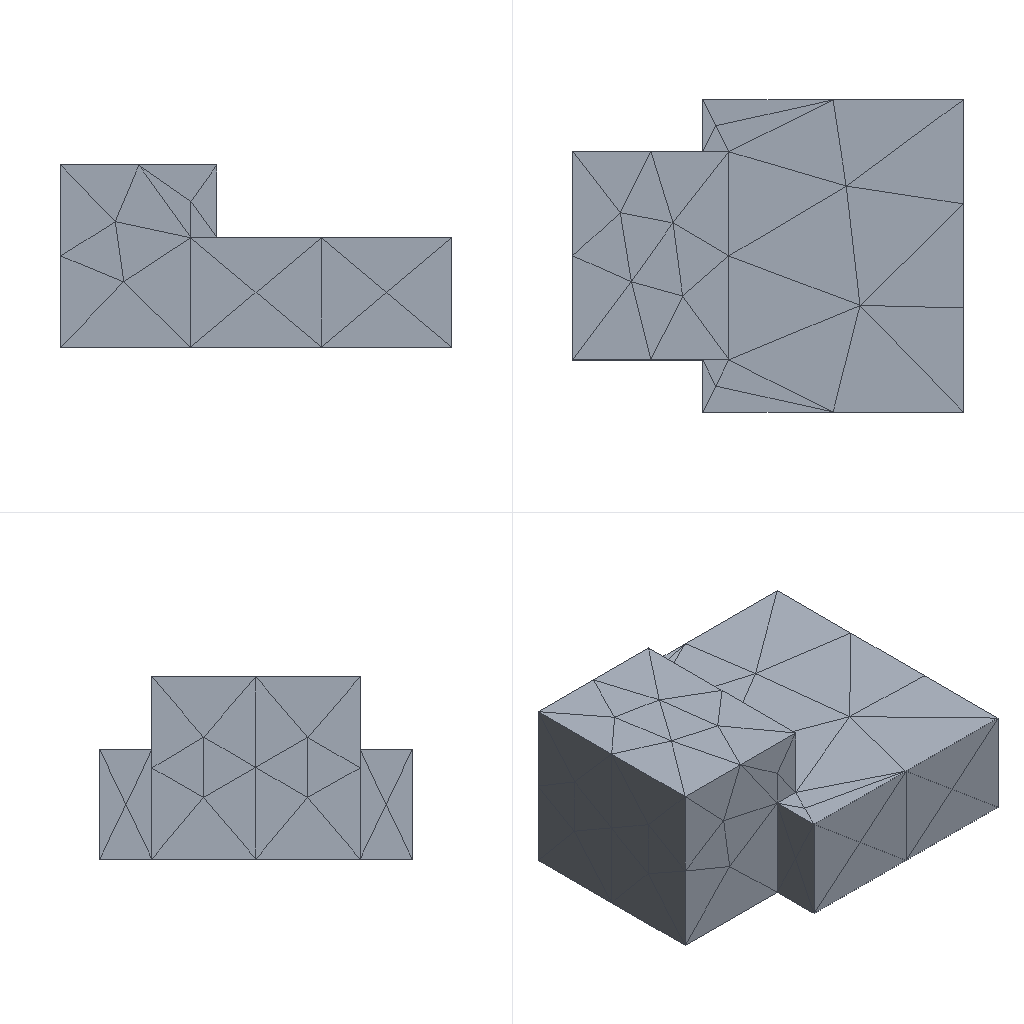Simulation study | ansys mapdl
Set-up summary:
category,name,step,type,value,unit,region
solver,ansys_mapdl
units,mm-N-s-tonne (MPa),,inferred,E=210000 density=
analysis,model,,static
mesh,nodes,,,484
mesh,elements,,,236
element_type,SOLID187,,,236
material,mat 1,,E,210000
material,mat 1,,nu,0.3
load,,model,body load temp,,,all
load,,model,force,"1000 [dir=(0, 0, -1) n=95]",,node list
bc,,model,fixed,"[dofs=UX,UY,UZ n=624]",,node list
Ansys APDL input file, long lists of numbers shortened:
/COM,ANSYS RELEASE 2026 R1           BUILD 26.1      UP20260202       09:10:16
/PREP7
/NOPR
/TITLE,2
ANTYPE, 0
*IF,_CDRDOFF,EQ,1,THEN     !if solid model was read in
_CDRDOFF=             !reset flag, numoffs already performed
*ELSE              !offset database for the following FE model
NUMOFF,NODE,      484
NUMOFF,ELEM,      236
NUMOFF,MAT ,        1
NUMOFF,TYPE,        1
*ENDIF
*SET,_RETURN ,  0.
*SET,_STATUS ,  0.
*SET,_UIQR   ,  95.
*SET,__FLOATPARAMETER__,  484.
DOF,DELETE
ETBLOCK,        1,        1
(2i9,19a9)
        1      187        0        0        0        0        0        0        0        0        0        0        0        0        0        0        0        0        0        0        0
       -1
NBLOCK,6,SOLID,       484,       484
(3i9,6e21.13e3)
        1        0        0 5.5000000000000E+001-1.2000000000000E+001
! (483 more lines like these left out)
N,UNBL,LOC,       -1,
EBLOCK,19,SOLID,       236,       236
(19i10)
         1         1         1         1         0         0         0         0        10         0         1       303       304        86       305       313       314       315       316
! (471 more lines like these left out)
        -1
MPTEMP,UNBL, 1, 1,  0.    ,
MPDATA,UNBL, 1,EX  ,       1, 1,  210000.000    ,
MPTEMP,UNBL, 1, 1,  0.    ,
MPDATA,UNBL, 1,NUXY,       1, 1, 0.3    ,
MPTEMP,UNBL, 1, 1,  0.    ,
MPDATA,UNBL, 1,PRXY,       1, 1, 0.3    ,
EXTOPT,ATTR,      0,      0,      0
EXTOPT,ESIZE,  0,  0.
EXTOPT,ACLEAR,      0
TREF,  0.
IRLF,  0
BFUNIF,TEMP,_TINY
ACEL,  0.    ,  0.    ,  0.
OMEGA,  0.    ,  0.    ,  0.
DOMEGA,  0.    ,  0.    ,  0.
CGLOC,  0.    ,  0.    ,  0.
CGOMEGA,  0.    ,  0.    ,  0.
DCGOMG,  0.    ,  0.    ,  0.
KUSE,     0
TIME,  0.
ALPHAD,  0.
BETAD,  0.
DMPRAT,  0.
DMPSTR,  0.
CRPLIM, 0.1    ,   0
CRPLIM,  0.    ,   1
NCNV,     0, 1.000000000E+12,     0,  0.    ,  0.
NEQIT,     0
ERESX,DEFA
DBLOCK,       624
(i9,a6,2(pg16.9))
        1  UX    0.00000000      0.00000000
! (623 more lines like these left out)
       -1
FBLOCK,        95
(i9,a6,2(pg16.9))
      188  FZ   -10.5263158      0.00000000
! (94 more lines like these left out)
       -1
/GO
FINISH
Results summary:
result,analysis_type_db,,,static,unstated
result,n_sets,,,1,unstated
result,load_steps[0].set,load_step=1,,1,unstated
result,load_steps[0].substep,load_step=1,,1,unstated
result,load_steps[0].time,load_step=1,,1,unstated
result,load_steps[0].freq,load_step=1,,1,unstated
result,load_steps[0].max_usum,load_step=1,,0.0004767,unstated
result,load_steps[0].max_seqv,load_step=1,,10.72,unstated
result,load_steps[0].reaction_sum.FX,load_step=1,,-1.21148e-11,unstated
result,load_steps[0].reaction_sum.FY,load_step=1,,-1.51772e-11,unstated
result,load_steps[0].reaction_sum.FZ,load_step=1,,1000,unstated
result,load_steps[0].reaction_sum.MX,load_step=1,,0,unstated
result,load_steps[0].reaction_sum.MY,load_step=1,,0,unstated
result,load_steps[0].reaction_sum.MZ,load_step=1,,0,unstated
result,convergence,,,results present for all listed sets,unstated